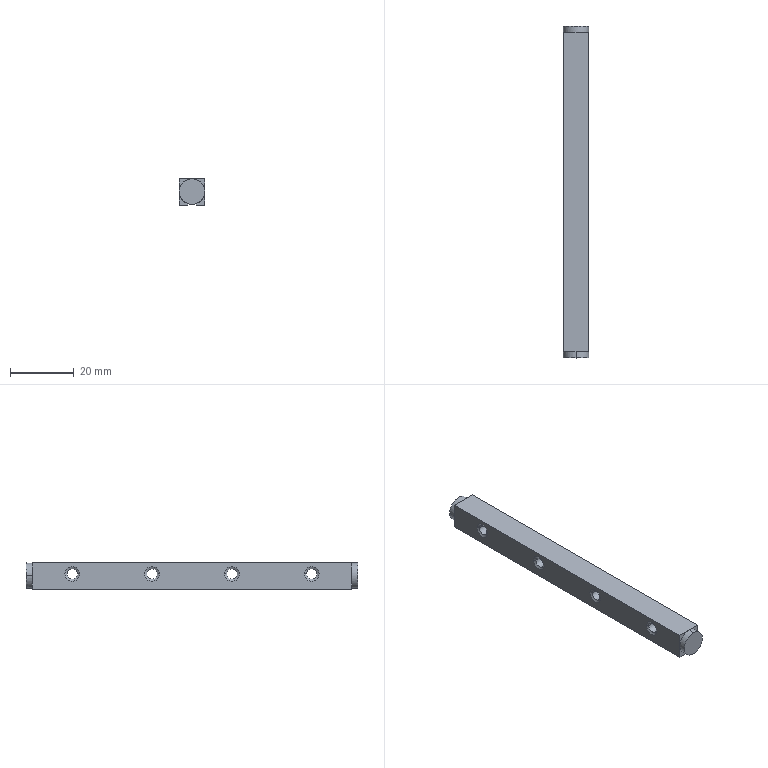Part | NX | 1 solid | 51 faces | box 8 x 104 x 8.3 mm | volume 6115 mm3 | plane 23 | cylinder 20 | cone 8 | commonest cylinder face diameters 3.3 x8 6 x8 8 x4
STEP:
#1=CARTESIAN_POINT('',(4.995,0.,-7.874));
#2=VERTEX_POINT('',#1);
#3=CARTESIAN_POINT('',(8.,0.,-4.));
#4=VERTEX_POINT('',#3);
#5=CARTESIAN_POINT('',(4.,0.,-4.));
#6=DIRECTION('',(0.,-1.,0.));
#7=DIRECTION('',(0.2489,0.,-0.9685));
#8=AXIS2_PLACEMENT_3D('',#5,#6,#7);
#9=CIRCLE('',#8,4.);
#10=EDGE_CURVE('',#2,#4,#9,.T.);
#11=ORIENTED_EDGE('',*,*,#10,.F.);
#12=CARTESIAN_POINT('',(5.421,0.,-8.3));
#13=VERTEX_POINT('',#12);
#14=CARTESIAN_POINT('',(5.421,0.,-8.3));
#15=DIRECTION('',(-0.7071,0.,0.7071));
#16=VECTOR('',#15,1000.);
#17=LINE('',#14,#16);
#18=EDGE_CURVE('',#13,#2,#17,.T.);
#19=ORIENTED_EDGE('',*,*,#18,.F.);
#20=CARTESIAN_POINT('',(8.,0.,-8.3));
#21=VERTEX_POINT('',#20);
#22=CARTESIAN_POINT('',(5.421,0.,-8.3));
#23=DIRECTION('',(1.,0.,0.));
#24=VECTOR('',#23,1000.);
#25=LINE('',#22,#24);
#26=EDGE_CURVE('',#13,#21,#25,.T.);
#27=ORIENTED_EDGE('',*,*,#26,.T.);
#28=CARTESIAN_POINT('',(8.,0.,-8.3));
#29=DIRECTION('',(0.,0.,1.));
#30=VECTOR('',#29,1000.);
#31=LINE('',#28,#30);
#32=EDGE_CURVE('',#21,#4,#31,.T.);
#33=ORIENTED_EDGE('',*,*,#32,.T.);
#34=EDGE_LOOP('',(#11,#19,#27,#33));
#35=FACE_BOUND('',#34,.T.);
#36=CARTESIAN_POINT('',(0.,0.,0.));
#37=DIRECTION('',(0.,1.,0.));
#38=DIRECTION('',(1.,0.,0.));
#39=AXIS2_PLACEMENT_3D('',#36,#37,#38);
#40=PLANE('',#39);
#41=ADVANCED_FACE('',(#35),#40,.F.);
#42=CARTESIAN_POINT('',(4.,-2.,0.));
#43=VERTEX_POINT('',#42);
#44=CARTESIAN_POINT('',(4.,-2.,-8.));
#45=VERTEX_POINT('',#44);
#46=CARTESIAN_POINT('',(4.,-2.,-4.));
#47=DIRECTION('',(0.,1.,0.));
#48=DIRECTION('',(0.,0.,1.));
#49=AXIS2_PLACEMENT_3D('',#46,#47,#48);
#50=CIRCLE('',#49,4.);
#51=EDGE_CURVE('',#43,#45,#50,.T.);
#52=ORIENTED_EDGE('',*,*,#51,.T.);
#53=CARTESIAN_POINT('',(4.,0.,-8.));
#54=VERTEX_POINT('',#53);
#55=CARTESIAN_POINT('',(4.,0.,-8.));
#56=DIRECTION('',(0.,-1.,0.));
#57=VECTOR('',#56,1000.);
#58=LINE('',#55,#57);
#59=EDGE_CURVE('',#45,#54,#58,.F.);
#60=ORIENTED_EDGE('',*,*,#59,.T.);
#61=CARTESIAN_POINT('',(4.,0.,-4.));
#62=DIRECTION('',(0.,-1.,0.));
#63=DIRECTION('',(-0.2489,0.,-0.9685));
#64=AXIS2_PLACEMENT_3D('',#61,#62,#63);
#65=CIRCLE('',#64,4.);
#66=EDGE_CURVE('',#54,#2,#65,.T.);
#67=ORIENTED_EDGE('',*,*,#66,.T.);
#68=ORIENTED_EDGE('',*,*,#10,.T.);
#69=CARTESIAN_POINT('',(4.,0.,0.));
#70=VERTEX_POINT('',#69);
#71=CARTESIAN_POINT('',(4.,0.,-4.));
#72=DIRECTION('',(0.,-1.,0.));
#73=DIRECTION('',(1.,0.,0.));
#74=AXIS2_PLACEMENT_3D('',#71,#72,#73);
#75=CIRCLE('',#74,4.);
#76=EDGE_CURVE('',#4,#70,#75,.T.);
#77=ORIENTED_EDGE('',*,*,#76,.T.);
#78=CARTESIAN_POINT('',(4.,0.,0.));
#79=DIRECTION('',(0.,-1.,0.));
#80=VECTOR('',#79,1000.);
#81=LINE('',#78,#80);
#82=EDGE_CURVE('',#43,#70,#81,.F.);
#83=ORIENTED_EDGE('',*,*,#82,.F.);
#84=EDGE_LOOP('',(#52,#60,#67,#68,#77,#83));
#85=FACE_BOUND('',#84,.T.);
#86=CARTESIAN_POINT('',(4.,0.,-4.));
#87=DIRECTION('',(0.,-1.,0.));
#88=DIRECTION('',(0.,0.,-1.));
#89=AXIS2_PLACEMENT_3D('',#86,#87,#88);
#90=CYLINDRICAL_SURFACE('',#89,4.);
#91=ADVANCED_FACE('',(#85),#90,.T.);
#92=CARTESIAN_POINT('',(4.,0.,-6.879));
#93=VERTEX_POINT('',#92);
#94=CARTESIAN_POINT('',(3.005,0.,-7.874));
#95=VERTEX_POINT('',#94);
#96=CARTESIAN_POINT('',(4.,0.,-6.879));
#97=DIRECTION('',(-0.7071,0.,-0.7071));
#98=VECTOR('',#97,1000.);
#99=LINE('',#96,#98);
#100=EDGE_CURVE('',#93,#95,#99,.T.);
#101=ORIENTED_EDGE('',*,*,#100,.F.);
#102=CARTESIAN_POINT('',(4.995,0.,-7.874));
#103=DIRECTION('',(-0.7071,0.,0.7071));
#104=VECTOR('',#103,1000.);
#105=LINE('',#102,#104);
#106=EDGE_CURVE('',#2,#93,#105,.T.);
#107=ORIENTED_EDGE('',*,*,#106,.F.);
#108=ORIENTED_EDGE('',*,*,#66,.F.);
#109=CARTESIAN_POINT('',(4.,0.,-4.));
#110=DIRECTION('',(0.,-1.,0.));
#111=DIRECTION('',(-0.2489,0.,-0.9685));
#112=AXIS2_PLACEMENT_3D('',#109,#110,#111);
#113=CIRCLE('',#112,4.);
#114=EDGE_CURVE('',#95,#54,#113,.T.);
#115=ORIENTED_EDGE('',*,*,#114,.F.);
#116=EDGE_LOOP('',(#101,#107,#108,#115));
#117=FACE_BOUND('',#116,.T.);
#118=CARTESIAN_POINT('',(0.,0.,0.));
#119=DIRECTION('',(0.,-1.,0.));
#120=DIRECTION('',(0.,0.,-1.));
#121=AXIS2_PLACEMENT_3D('',#118,#119,#120);
#122=PLANE('',#121);
#123=ADVANCED_FACE('',(#117),#122,.F.);
#124=ORIENTED_EDGE('',*,*,#100,.T.);
#125=CARTESIAN_POINT('',(2.579,0.,-8.3));
#126=VERTEX_POINT('',#125);
#127=CARTESIAN_POINT('',(3.005,0.,-7.874));
#128=DIRECTION('',(-0.7071,0.,-0.7071));
#129=VECTOR('',#128,1000.);
#130=LINE('',#127,#129);
#131=EDGE_CURVE('',#95,#126,#130,.T.);
#132=ORIENTED_EDGE('',*,*,#131,.T.);
#133=CARTESIAN_POINT('',(2.579,100.,-8.3));
#134=VERTEX_POINT('',#133);
#135=CARTESIAN_POINT('',(2.579,100.,-8.3));
#136=DIRECTION('',(0.,-1.,0.));
#137=VECTOR('',#136,1000.);
#138=LINE('',#135,#137);
#139=EDGE_CURVE('',#134,#126,#138,.T.);
#140=ORIENTED_EDGE('',*,*,#139,.F.);
#141=CARTESIAN_POINT('',(3.005,100.,-7.874));
#142=VERTEX_POINT('',#141);
#143=CARTESIAN_POINT('',(2.579,100.,-8.3));
#144=DIRECTION('',(0.7071,0.,0.7071));
#145=VECTOR('',#144,1000.);
#146=LINE('',#143,#145);
#147=EDGE_CURVE('',#134,#142,#146,.T.);
#148=ORIENTED_EDGE('',*,*,#147,.T.);
#149=CARTESIAN_POINT('',(4.,100.,-6.879));
#150=VERTEX_POINT('',#149);
#151=CARTESIAN_POINT('',(3.005,100.,-7.874));
#152=DIRECTION('',(0.7071,0.,0.7071));
#153=VECTOR('',#152,1000.);
#154=LINE('',#151,#153);
#155=EDGE_CURVE('',#142,#150,#154,.T.);
#156=ORIENTED_EDGE('',*,*,#155,.T.);
#157=CARTESIAN_POINT('',(4.,0.,-6.879));
#158=DIRECTION('',(0.,1.,0.));
#159=VECTOR('',#158,1000.);
#160=LINE('',#157,#159);
#161=EDGE_CURVE('',#93,#150,#160,.T.);
#162=ORIENTED_EDGE('',*,*,#161,.F.);
#163=EDGE_LOOP('',(#124,#132,#140,#148,#156,#162));
#164=FACE_BOUND('',#163,.T.);
#165=CARTESIAN_POINT('',(1.879,100.,-9.));
#166=DIRECTION('',(-0.7071,0.,0.7071));
#167=DIRECTION('',(0.,1.,0.));
#168=AXIS2_PLACEMENT_3D('',#165,#166,#167);
#169=PLANE('',#168);
#170=ADVANCED_FACE('',(#164),#169,.F.);
#171=ORIENTED_EDGE('',*,*,#106,.T.);
#172=ORIENTED_EDGE('',*,*,#161,.T.);
#173=CARTESIAN_POINT('',(4.995,100.,-7.874));
#174=VERTEX_POINT('',#173);
#175=CARTESIAN_POINT('',(4.,100.,-6.879));
#176=DIRECTION('',(0.7071,0.,-0.7071));
#177=VECTOR('',#176,1000.);
#178=LINE('',#175,#177);
#179=EDGE_CURVE('',#150,#174,#178,.T.);
#180=ORIENTED_EDGE('',*,*,#179,.T.);
#181=CARTESIAN_POINT('',(5.421,100.,-8.3));
#182=VERTEX_POINT('',#181);
#183=CARTESIAN_POINT('',(4.995,100.,-7.874));
#184=DIRECTION('',(0.7071,0.,-0.7071));
#185=VECTOR('',#184,1000.);
#186=LINE('',#183,#185);
#187=EDGE_CURVE('',#174,#182,#186,.T.);
#188=ORIENTED_EDGE('',*,*,#187,.T.);
#189=CARTESIAN_POINT('',(5.421,100.,-8.3));
#190=DIRECTION('',(0.,-1.,0.));
#191=VECTOR('',#190,1000.);
#192=LINE('',#189,#191);
#193=EDGE_CURVE('',#182,#13,#192,.T.);
#194=ORIENTED_EDGE('',*,*,#193,.T.);
#195=ORIENTED_EDGE('',*,*,#18,.T.);
#196=EDGE_LOOP('',(#171,#172,#180,#188,#194,#195));
#197=FACE_BOUND('',#196,.T.);
#198=CARTESIAN_POINT('',(4.,100.,-6.879));
#199=DIRECTION('',(0.7071,0.,0.7071));
#200=DIRECTION('',(0.,-1.,0.));
#201=AXIS2_PLACEMENT_3D('',#198,#199,#200);
#202=PLANE('',#201);
#203=ADVANCED_FACE('',(#197),#202,.F.);
#204=ORIENTED_EDGE('',*,*,#193,.F.);
#205=CARTESIAN_POINT('',(8.,100.,-8.3));
#206=VERTEX_POINT('',#205);
#207=CARTESIAN_POINT('',(5.421,100.,-8.3));
#208=DIRECTION('',(1.,0.,0.));
#209=VECTOR('',#208,1000.);
#210=LINE('',#207,#209);
#211=EDGE_CURVE('',#182,#206,#210,.T.);
#212=ORIENTED_EDGE('',*,*,#211,.T.);
#213=CARTESIAN_POINT('',(8.,100.,-8.3));
#214=DIRECTION('',(0.,-1.,0.));
#215=VECTOR('',#214,1000.);
#216=LINE('',#213,#215);
#217=EDGE_CURVE('',#206,#21,#216,.T.);
#218=ORIENTED_EDGE('',*,*,#217,.T.);
#219=ORIENTED_EDGE('',*,*,#26,.F.);
#220=EDGE_LOOP('',(#204,#212,#218,#219));
#221=FACE_BOUND('',#220,.T.);
#222=CARTESIAN_POINT('',(8.,0.,-8.3));
#223=DIRECTION('',(0.,0.,-1.));
#224=DIRECTION('',(0.,-1.,0.));
#225=AXIS2_PLACEMENT_3D('',#222,#223,#224);
#226=PLANE('',#225);
#227=ADVANCED_FACE('',(#221),#226,.T.);
#228=CARTESIAN_POINT('',(8.,0.,0.));
#229=VERTEX_POINT('',#228);
#230=CARTESIAN_POINT('',(8.,0.,-4.));
#231=DIRECTION('',(0.,0.,1.));
#232=VECTOR('',#231,1000.);
#233=LINE('',#230,#232);
#234=EDGE_CURVE('',#4,#229,#233,.T.);
#235=ORIENTED_EDGE('',*,*,#234,.F.);
#236=ORIENTED_EDGE('',*,*,#32,.F.);
#237=ORIENTED_EDGE('',*,*,#217,.F.);
#238=CARTESIAN_POINT('',(8.,100.,-4.));
#239=VERTEX_POINT('',#238);
#240=CARTESIAN_POINT('',(8.,100.,-8.3));
#241=DIRECTION('',(0.,0.,1.));
#242=VECTOR('',#241,1000.);
#243=LINE('',#240,#242);
#244=EDGE_CURVE('',#206,#239,#243,.T.);
#245=ORIENTED_EDGE('',*,*,#244,.T.);
#246=CARTESIAN_POINT('',(8.,100.,0.));
#247=VERTEX_POINT('',#246);
#248=CARTESIAN_POINT('',(8.,100.,-4.));
#249=DIRECTION('',(0.,0.,1.));
#250=VECTOR('',#249,1000.);
#251=LINE('',#248,#250);
#252=EDGE_CURVE('',#239,#247,#251,.T.);
#253=ORIENTED_EDGE('',*,*,#252,.T.);
#254=CARTESIAN_POINT('',(8.,100.,0.));
#255=DIRECTION('',(0.,-1.,0.));
#256=VECTOR('',#255,1000.);
#257=LINE('',#254,#256);
#258=EDGE_CURVE('',#247,#229,#257,.T.);
#259=ORIENTED_EDGE('',*,*,#258,.T.);
#260=EDGE_LOOP('',(#235,#236,#237,#245,#253,#259));
#261=FACE_BOUND('',#260,.T.);
#262=CARTESIAN_POINT('',(8.,84.5,-3.5));
#263=VERTEX_POINT('',#262);
#264=CARTESIAN_POINT('',(8.,90.5,-3.5));
#265=VERTEX_POINT('',#264);
#266=CARTESIAN_POINT('',(8.,87.5,-3.5));
#267=DIRECTION('',(1.,0.,0.));
#268=DIRECTION('',(0.,1.,0.));
#269=AXIS2_PLACEMENT_3D('',#266,#267,#268);
#270=CIRCLE('',#269,3.);
#271=EDGE_CURVE('',#263,#265,#270,.T.);
#272=ORIENTED_EDGE('',*,*,#271,.F.);
#273=CARTESIAN_POINT('',(8.,87.5,-3.5));
#274=DIRECTION('',(1.,0.,0.));
#275=DIRECTION('',(0.,1.,0.));
#276=AXIS2_PLACEMENT_3D('',#273,#274,#275);
#277=CIRCLE('',#276,3.);
#278=EDGE_CURVE('',#265,#263,#277,.T.);
#279=ORIENTED_EDGE('',*,*,#278,.F.);
#280=EDGE_LOOP('',(#272,#279));
#281=FACE_BOUND('',#280,.T.);
#282=CARTESIAN_POINT('',(8.,59.5,-3.5));
#283=VERTEX_POINT('',#282);
#284=CARTESIAN_POINT('',(8.,65.5,-3.5));
#285=VERTEX_POINT('',#284);
#286=CARTESIAN_POINT('',(8.,62.5,-3.5));
#287=DIRECTION('',(1.,0.,0.));
#288=DIRECTION('',(0.,1.,0.));
#289=AXIS2_PLACEMENT_3D('',#286,#287,#288);
#290=CIRCLE('',#289,3.);
#291=EDGE_CURVE('',#283,#285,#290,.T.);
#292=ORIENTED_EDGE('',*,*,#291,.F.);
#293=CARTESIAN_POINT('',(8.,62.5,-3.5));
#294=DIRECTION('',(1.,0.,0.));
#295=DIRECTION('',(0.,1.,0.));
#296=AXIS2_PLACEMENT_3D('',#293,#294,#295);
#297=CIRCLE('',#296,3.);
#298=EDGE_CURVE('',#285,#283,#297,.T.);
#299=ORIENTED_EDGE('',*,*,#298,.F.);
#300=EDGE_LOOP('',(#292,#299));
#301=FACE_BOUND('',#300,.T.);
#302=CARTESIAN_POINT('',(8.,40.5,-3.5));
#303=VERTEX_POINT('',#302);
#304=CARTESIAN_POINT('',(8.,34.5,-3.5));
#305=VERTEX_POINT('',#304);
#306=CARTESIAN_POINT('',(8.,37.5,-3.5));
#307=DIRECTION('',(1.,0.,0.));
#308=DIRECTION('',(0.,1.,0.));
#309=AXIS2_PLACEMENT_3D('',#306,#307,#308);
#310=CIRCLE('',#309,3.);
#311=EDGE_CURVE('',#303,#305,#310,.T.);
#312=ORIENTED_EDGE('',*,*,#311,.F.);
#313=CARTESIAN_POINT('',(8.,37.5,-3.5));
#314=DIRECTION('',(1.,0.,0.));
#315=DIRECTION('',(0.,1.,0.));
#316=AXIS2_PLACEMENT_3D('',#313,#314,#315);
#317=CIRCLE('',#316,3.);
#318=EDGE_CURVE('',#305,#303,#317,.T.);
#319=ORIENTED_EDGE('',*,*,#318,.F.);
#320=EDGE_LOOP('',(#312,#319));
#321=FACE_BOUND('',#320,.T.);
#322=CARTESIAN_POINT('',(8.,15.5,-3.5));
#323=VERTEX_POINT('',#322);
#324=CARTESIAN_POINT('',(8.,9.5,-3.5));
#325=VERTEX_POINT('',#324);
#326=CARTESIAN_POINT('',(8.,12.5,-3.5));
#327=DIRECTION('',(1.,0.,0.));
#328=DIRECTION('',(0.,1.,0.));
#329=AXIS2_PLACEMENT_3D('',#326,#327,#328);
#330=CIRCLE('',#329,3.);
#331=EDGE_CURVE('',#323,#325,#330,.T.);
#332=ORIENTED_EDGE('',*,*,#331,.F.);
#333=CARTESIAN_POINT('',(8.,12.5,-3.5));
#334=DIRECTION('',(1.,0.,0.));
#335=DIRECTION('',(0.,1.,0.));
#336=AXIS2_PLACEMENT_3D('',#333,#334,#335);
#337=CIRCLE('',#336,3.);
#338=EDGE_CURVE('',#325,#323,#337,.T.);
#339=ORIENTED_EDGE('',*,*,#338,.F.);
#340=EDGE_LOOP('',(#332,#339));
#341=FACE_BOUND('',#340,.T.);
#342=CARTESIAN_POINT('',(8.,0.,0.));
#343=DIRECTION('',(1.,0.,0.));
#344=DIRECTION('',(0.,1.,0.));
#345=AXIS2_PLACEMENT_3D('',#342,#343,#344);
#346=PLANE('',#345);
#347=ADVANCED_FACE('',(#261,#281,#301,#321,#341),#346,.T.);
#348=ORIENTED_EDGE('',*,*,#76,.F.);
#349=ORIENTED_EDGE('',*,*,#234,.T.);
#350=CARTESIAN_POINT('',(8.,0.,0.));
#351=DIRECTION('',(-1.,0.,0.));
#352=VECTOR('',#351,1000.);
#353=LINE('',#350,#352);
#354=EDGE_CURVE('',#229,#70,#353,.T.);
#355=ORIENTED_EDGE('',*,*,#354,.T.);
#356=EDGE_LOOP('',(#348,#349,#355));
#357=FACE_BOUND('',#356,.T.);
#358=CARTESIAN_POINT('',(0.,0.,0.));
#359=DIRECTION('',(0.,1.,0.));
#360=DIRECTION('',(1.,0.,0.));
#361=AXIS2_PLACEMENT_3D('',#358,#359,#360);
#362=PLANE('',#361);
#363=ADVANCED_FACE('',(#357),#362,.F.);
#364=CARTESIAN_POINT('',(0.,0.,0.));
#365=VERTEX_POINT('',#364);
#366=CARTESIAN_POINT('',(4.,0.,0.));
#367=DIRECTION('',(-1.,0.,0.));
#368=VECTOR('',#367,1000.);
#369=LINE('',#366,#368);
#370=EDGE_CURVE('',#70,#365,#369,.T.);
#371=ORIENTED_EDGE('',*,*,#370,.F.);
#372=ORIENTED_EDGE('',*,*,#354,.F.);
#373=ORIENTED_EDGE('',*,*,#258,.F.);
#374=CARTESIAN_POINT('',(4.,100.,0.));
#375=VERTEX_POINT('',#374);
#376=CARTESIAN_POINT('',(8.,100.,0.));
#377=DIRECTION('',(-1.,0.,0.));
#378=VECTOR('',#377,1000.);
#379=LINE('',#376,#378);
#380=EDGE_CURVE('',#247,#375,#379,.T.);
#381=ORIENTED_EDGE('',*,*,#380,.T.);
#382=CARTESIAN_POINT('',(0.,100.,0.));
#383=VERTEX_POINT('',#382);
#384=CARTESIAN_POINT('',(4.,100.,0.));
#385=DIRECTION('',(-1.,0.,0.));
#386=VECTOR('',#385,1000.);
#387=LINE('',#384,#386);
#388=EDGE_CURVE('',#375,#383,#387,.T.);
#389=ORIENTED_EDGE('',*,*,#388,.T.);
#390=CARTESIAN_POINT('',(0.,0.,0.));
#391=DIRECTION('',(0.,-1.,0.));
#392=VECTOR('',#391,1000.);
#393=LINE('',#390,#392);
#394=EDGE_CURVE('',#383,#365,#393,.T.);
#395=ORIENTED_EDGE('',*,*,#394,.T.);
#396=EDGE_LOOP('',(#371,#372,#373,#381,#389,#395));
#397=FACE_BOUND('',#396,.T.);
#398=CARTESIAN_POINT('',(0.,0.,0.));
#399=DIRECTION('',(0.,0.,1.));
#400=DIRECTION('',(1.,0.,0.));
#401=AXIS2_PLACEMENT_3D('',#398,#399,#400);
#402=PLANE('',#401);
#403=ADVANCED_FACE('',(#397),#402,.T.);
#404=CARTESIAN_POINT('',(0.,0.,-4.));
#405=VERTEX_POINT('',#404);
#406=CARTESIAN_POINT('',(4.,0.,-4.));
#407=DIRECTION('',(0.,-1.,0.));
#408=DIRECTION('',(0.,0.,1.));
#409=AXIS2_PLACEMENT_3D('',#406,#407,#408);
#410=CIRCLE('',#409,4.);
#411=EDGE_CURVE('',#70,#405,#410,.T.);
#412=ORIENTED_EDGE('',*,*,#411,.F.);
#413=ORIENTED_EDGE('',*,*,#370,.T.);
#414=CARTESIAN_POINT('',(0.,0.,0.));
#415=DIRECTION('',(0.,0.,1.));
#416=VECTOR('',#415,1000.);
#417=LINE('',#414,#416);
#418=EDGE_CURVE('',#405,#365,#417,.T.);
#419=ORIENTED_EDGE('',*,*,#418,.F.);
#420=EDGE_LOOP('',(#412,#413,#419));
#421=FACE_BOUND('',#420,.T.);
#422=CARTESIAN_POINT('',(0.,0.,0.));
#423=DIRECTION('',(0.,1.,0.));
#424=DIRECTION('',(1.,0.,0.));
#425=AXIS2_PLACEMENT_3D('',#422,#423,#424);
#426=PLANE('',#425);
#427=ADVANCED_FACE('',(#421),#426,.F.);
#428=CARTESIAN_POINT('',(4.9,15.5,-3.5));
#429=VERTEX_POINT('',#428);
#430=CARTESIAN_POINT('',(4.9,9.5,-3.5));
#431=VERTEX_POINT('',#430);
#432=CARTESIAN_POINT('',(4.9,12.5,-3.5));
#433=DIRECTION('',(1.,0.,0.));
#434=DIRECTION('',(0.,-1.,0.));
#435=AXIS2_PLACEMENT_3D('',#432,#433,#434);
#436=CIRCLE('',#435,3.);
#437=EDGE_CURVE('',#429,#431,#436,.T.);
#438=ORIENTED_EDGE('',*,*,#437,.T.);
#439=CARTESIAN_POINT('',(4.9,12.5,-3.5));
#440=DIRECTION('',(1.,0.,0.));
#441=DIRECTION('',(0.,-1.,0.));
#442=AXIS2_PLACEMENT_3D('',#439,#440,#441);
#443=CIRCLE('',#442,3.);
#444=EDGE_CURVE('',#431,#429,#443,.T.);
#445=ORIENTED_EDGE('',*,*,#444,.T.);
#446=EDGE_LOOP('',(#438,#445));
#447=FACE_BOUND('',#446,.T.);
#448=CARTESIAN_POINT('',(4.9,14.15,-3.5));
#449=VERTEX_POINT('',#448);
#450=CARTESIAN_POINT('',(4.9,10.85,-3.5));
#451=VERTEX_POINT('',#450);
#452=CARTESIAN_POINT('',(4.9,12.5,-3.5));
#453=DIRECTION('',(-1.,0.,0.));
#454=DIRECTION('',(0.,1.,0.));
#455=AXIS2_PLACEMENT_3D('',#452,#453,#454);
#456=CIRCLE('',#455,1.65);
#457=EDGE_CURVE('',#449,#451,#456,.T.);
#458=ORIENTED_EDGE('',*,*,#457,.T.);
#459=CARTESIAN_POINT('',(4.9,12.5,-3.5));
#460=DIRECTION('',(-1.,0.,0.));
#461=DIRECTION('',(0.,1.,0.));
#462=AXIS2_PLACEMENT_3D('',#459,#460,#461);
#463=CIRCLE('',#462,1.65);
#464=EDGE_CURVE('',#451,#449,#463,.T.);
#465=ORIENTED_EDGE('',*,*,#464,.T.);
#466=EDGE_LOOP('',(#458,#465));
#467=FACE_BOUND('',#466,.T.);
#468=CARTESIAN_POINT('',(4.9,12.5,-3.5));
#469=DIRECTION('',(1.,0.,0.));
#470=DIRECTION('',(0.,1.,0.));
#471=AXIS2_PLACEMENT_3D('',#468,#469,#470);
#472=PLANE('',#471);
#473=ADVANCED_FACE('',(#447,#467),#472,.T.);
#474=ORIENTED_EDGE('',*,*,#51,.F.);
#475=CARTESIAN_POINT('',(4.,-2.,-4.));
#476=DIRECTION('',(0.,1.,0.));
#477=DIRECTION('',(0.,0.,1.));
#478=AXIS2_PLACEMENT_3D('',#475,#476,#477);
#479=CIRCLE('',#478,4.);
#480=EDGE_CURVE('',#45,#43,#479,.T.);
#481=ORIENTED_EDGE('',*,*,#480,.F.);
#482=EDGE_LOOP('',(#474,#481));
#483=FACE_BOUND('',#482,.T.);
#484=CARTESIAN_POINT('',(0.,-2.,0.));
#485=DIRECTION('',(0.,-1.,0.));
#486=DIRECTION('',(0.,0.,-1.));
#487=AXIS2_PLACEMENT_3D('',#484,#485,#486);
#488=PLANE('',#487);
#489=ADVANCED_FACE('',(#483),#488,.T.);
#490=CARTESIAN_POINT('',(4.,0.,-4.));
#491=DIRECTION('',(0.,-1.,0.));
#492=DIRECTION('',(-1.,0.,0.));
#493=AXIS2_PLACEMENT_3D('',#490,#491,#492);
#494=CIRCLE('',#493,4.);
#495=EDGE_CURVE('',#405,#95,#494,.T.);
#496=ORIENTED_EDGE('',*,*,#495,.F.);
#497=CARTESIAN_POINT('',(0.,0.,-8.3));
#498=VERTEX_POINT('',#497);
#499=CARTESIAN_POINT('',(0.,0.,0.));
#500=DIRECTION('',(0.,0.,1.));
#501=VECTOR('',#500,1000.);
#502=LINE('',#499,#501);
#503=EDGE_CURVE('',#498,#405,#502,.T.);
#504=ORIENTED_EDGE('',*,*,#503,.F.);
#505=CARTESIAN_POINT('',(0.,0.,-8.3));
#506=DIRECTION('',(1.,0.,0.));
#507=VECTOR('',#506,1000.);
#508=LINE('',#505,#507);
#509=EDGE_CURVE('',#498,#126,#508,.T.);
#510=ORIENTED_EDGE('',*,*,#509,.T.);
#511=ORIENTED_EDGE('',*,*,#131,.F.);
#512=EDGE_LOOP('',(#496,#504,#510,#511));
#513=FACE_BOUND('',#512,.T.);
#514=CARTESIAN_POINT('',(0.,0.,0.));
#515=DIRECTION('',(0.,1.,0.));
#516=DIRECTION('',(1.,0.,0.));
#517=AXIS2_PLACEMENT_3D('',#514,#515,#516);
#518=PLANE('',#517);
#519=ADVANCED_FACE('',(#513),#518,.F.);
#520=ORIENTED_EDGE('',*,*,#139,.T.);
#521=ORIENTED_EDGE('',*,*,#509,.F.);
#522=CARTESIAN_POINT('',(0.,100.,-8.3));
#523=VERTEX_POINT('',#522);
#524=CARTESIAN_POINT('',(0.,0.,-8.3));
#525=DIRECTION('',(0.,1.,0.));
#526=VECTOR('',#525,1000.);
#527=LINE('',#524,#526);
#528=EDGE_CURVE('',#498,#523,#527,.T.);
#529=ORIENTED_EDGE('',*,*,#528,.T.);
#530=CARTESIAN_POINT('',(0.,100.,-8.3));
#531=DIRECTION('',(1.,0.,0.));
#532=VECTOR('',#531,1000.);
#533=LINE('',#530,#532);
#534=EDGE_CURVE('',#523,#134,#533,.T.);
#535=ORIENTED_EDGE('',*,*,#534,.T.);
#536=EDGE_LOOP('',(#520,#521,#529,#535));
#537=FACE_BOUND('',#536,.T.);
#538=CARTESIAN_POINT('',(8.,0.,-8.3));
#539=DIRECTION('',(0.,0.,-1.));
#540=DIRECTION('',(0.,-1.,0.));
#541=AXIS2_PLACEMENT_3D('',#538,#539,#540);
#542=PLANE('',#541);
#543=ADVANCED_FACE('',(#537),#542,.T.);
#544=CARTESIAN_POINT('',(0.,100.,-4.));
#545=VERTEX_POINT('',#544);
#546=CARTESIAN_POINT('',(4.,100.,-4.));
#547=DIRECTION('',(0.,1.,0.));
#548=DIRECTION('',(-0.2489,0.,-0.9685));
#549=AXIS2_PLACEMENT_3D('',#546,#547,#548);
#550=CIRCLE('',#549,4.);
#551=EDGE_CURVE('',#142,#545,#550,.T.);
#552=ORIENTED_EDGE('',*,*,#551,.F.);
#553=ORIENTED_EDGE('',*,*,#147,.F.);
#554=ORIENTED_EDGE('',*,*,#534,.F.);
#555=CARTESIAN_POINT('',(0.,100.,0.));
#556=DIRECTION('',(0.,0.,1.));
#557=VECTOR('',#556,1000.);
#558=LINE('',#555,#557);
#559=EDGE_CURVE('',#523,#545,#558,.T.);
#560=ORIENTED_EDGE('',*,*,#559,.T.);
#561=EDGE_LOOP('',(#552,#553,#554,#560));
#562=FACE_BOUND('',#561,.T.);
#563=CARTESIAN_POINT('',(0.,100.,0.));
#564=DIRECTION('',(0.,1.,0.));
#565=DIRECTION('',(1.,0.,0.));
#566=AXIS2_PLACEMENT_3D('',#563,#564,#565);
#567=PLANE('',#566);
#568=ADVANCED_FACE('',(#562),#567,.T.);
#569=CARTESIAN_POINT('',(8.,102.,-4.));
#570=VERTEX_POINT('',#569);
#571=CARTESIAN_POINT('',(0.,102.,-4.));
#572=VERTEX_POINT('',#571);
#573=CARTESIAN_POINT('',(4.,102.,-4.));
#574=DIRECTION('',(0.,-1.,0.));
#575=DIRECTION('',(1.,0.,0.));
#576=AXIS2_PLACEMENT_3D('',#573,#574,#575);
#577=CIRCLE('',#576,4.);
#578=EDGE_CURVE('',#570,#572,#577,.T.);
#579=ORIENTED_EDGE('',*,*,#578,.T.);
#580=CARTESIAN_POINT('',(0.,100.,-4.));
#581=DIRECTION('',(0.,1.,0.));
#582=VECTOR('',#581,1000.);
#583=LINE('',#580,#582);
#584=EDGE_CURVE('',#572,#545,#583,.F.);
#585=ORIENTED_EDGE('',*,*,#584,.T.);
#586=CARTESIAN_POINT('',(4.,100.,-4.));
#587=DIRECTION('',(0.,1.,0.));
#588=DIRECTION('',(-1.,0.,0.));
#589=AXIS2_PLACEMENT_3D('',#586,#587,#588);
#590=CIRCLE('',#589,4.);
#591=EDGE_CURVE('',#545,#375,#590,.T.);
#592=ORIENTED_EDGE('',*,*,#591,.T.);
#593=CARTESIAN_POINT('',(4.,100.,-4.));
#594=DIRECTION('',(0.,1.,0.));
#595=DIRECTION('',(0.,0.,1.));
#596=AXIS2_PLACEMENT_3D('',#593,#594,#595);
#597=CIRCLE('',#596,4.);
#598=EDGE_CURVE('',#375,#239,#597,.T.);
#599=ORIENTED_EDGE('',*,*,#598,.T.);
#600=CARTESIAN_POINT('',(8.,100.,-4.));
#601=DIRECTION('',(0.,1.,0.));
#602=VECTOR('',#601,1000.);
#603=LINE('',#600,#602);
#604=EDGE_CURVE('',#570,#239,#603,.F.);
#605=ORIENTED_EDGE('',*,*,#604,.F.);
#606=EDGE_LOOP('',(#579,#585,#592,#599,#605));
#607=FACE_BOUND('',#606,.T.);
#608=CARTESIAN_POINT('',(4.,100.,-4.));
#609=DIRECTION('',(0.,1.,0.));
#610=DIRECTION('',(-1.,0.,0.));
#611=AXIS2_PLACEMENT_3D('',#608,#609,#610);
#612=CYLINDRICAL_SURFACE('',#611,4.);
#613=ADVANCED_FACE('',(#607),#612,.T.);
#614=CARTESIAN_POINT('',(4.,100.,-4.));
#615=DIRECTION('',(0.,1.,0.));
#616=DIRECTION('',(1.,0.,0.));
#617=AXIS2_PLACEMENT_3D('',#614,#615,#616);
#618=CIRCLE('',#617,4.);
#619=EDGE_CURVE('',#239,#174,#618,.T.);
#620=ORIENTED_EDGE('',*,*,#619,.F.);
#621=ORIENTED_EDGE('',*,*,#244,.F.);
#622=ORIENTED_EDGE('',*,*,#211,.F.);
#623=ORIENTED_EDGE('',*,*,#187,.F.);
#624=EDGE_LOOP('',(#620,#621,#622,#623));
#625=FACE_BOUND('',#624,.T.);
#626=CARTESIAN_POINT('',(0.,100.,0.));
#627=DIRECTION('',(0.,1.,0.));
#628=DIRECTION('',(1.,0.,0.));
#629=AXIS2_PLACEMENT_3D('',#626,#627,#628);
#630=PLANE('',#629);
#631=ADVANCED_FACE('',(#625),#630,.T.);
#632=CARTESIAN_POINT('',(4.9,40.5,-3.5));
#633=VERTEX_POINT('',#632);
#634=CARTESIAN_POINT('',(4.9,34.5,-3.5));
#635=VERTEX_POINT('',#634);
#636=CARTESIAN_POINT('',(4.9,37.5,-3.5));
#637=DIRECTION('',(1.,0.,0.));
#638=DIRECTION('',(0.,-1.,0.));
#639=AXIS2_PLACEMENT_3D('',#636,#637,#638);
#640=CIRCLE('',#639,3.);
#641=EDGE_CURVE('',#633,#635,#640,.T.);
#642=ORIENTED_EDGE('',*,*,#641,.F.);
#643=CARTESIAN_POINT('',(-1.24,40.5,-3.5));
#644=DIRECTION('',(1.,0.,0.));
#645=VECTOR('',#644,1000.);
#646=LINE('',#643,#645);
#647=EDGE_CURVE('',#303,#633,#646,.F.);
#648=ORIENTED_EDGE('',*,*,#647,.F.);
#649=ORIENTED_EDGE('',*,*,#311,.T.);
#650=CARTESIAN_POINT('',(-1.24,34.5,-3.5));
#651=DIRECTION('',(1.,0.,0.));
#652=VECTOR('',#651,1000.);
#653=LINE('',#650,#652);
#654=EDGE_CURVE('',#305,#635,#653,.F.);
#655=ORIENTED_EDGE('',*,*,#654,.T.);
#656=EDGE_LOOP('',(#642,#648,#649,#655));
#657=FACE_BOUND('',#656,.T.);
#658=CARTESIAN_POINT('',(-1.24,37.5,-3.5));
#659=DIRECTION('',(1.,0.,0.));
#660=DIRECTION('',(0.,-1.,0.));
#661=AXIS2_PLACEMENT_3D('',#658,#659,#660);
#662=CYLINDRICAL_SURFACE('',#661,3.);
#663=ADVANCED_FACE('',(#657),#662,.F.);
#664=ORIENTED_EDGE('',*,*,#591,.F.);
#665=CARTESIAN_POINT('',(0.,100.,0.));
#666=DIRECTION('',(0.,0.,1.));
#667=VECTOR('',#666,1000.);
#668=LINE('',#665,#667);
#669=EDGE_CURVE('',#545,#383,#668,.T.);
#670=ORIENTED_EDGE('',*,*,#669,.T.);
#671=ORIENTED_EDGE('',*,*,#388,.F.);
#672=EDGE_LOOP('',(#664,#670,#671));
#673=FACE_BOUND('',#672,.T.);
#674=CARTESIAN_POINT('',(0.,100.,0.));
#675=DIRECTION('',(0.,1.,0.));
#676=DIRECTION('',(1.,0.,0.));
#677=AXIS2_PLACEMENT_3D('',#674,#675,#676);
#678=PLANE('',#677);
#679=ADVANCED_FACE('',(#673),#678,.T.);
#680=ORIENTED_EDGE('',*,*,#503,.T.);
#681=ORIENTED_EDGE('',*,*,#418,.T.);
#682=ORIENTED_EDGE('',*,*,#394,.F.);
#683=ORIENTED_EDGE('',*,*,#669,.F.);
#684=ORIENTED_EDGE('',*,*,#559,.F.);
#685=ORIENTED_EDGE('',*,*,#528,.F.);
#686=EDGE_LOOP('',(#680,#681,#682,#683,#684,#685));
#687=FACE_BOUND('',#686,.T.);
#688=CARTESIAN_POINT('',(0.,10.185,-3.5));
#689=VERTEX_POINT('',#688);
#690=CARTESIAN_POINT('',(0.,14.815,-3.5));
#691=VERTEX_POINT('',#690);
#692=CARTESIAN_POINT('',(0.,12.5,-3.5));
#693=DIRECTION('',(-1.,0.,0.));
#694=DIRECTION('',(0.,1.,0.));
#695=AXIS2_PLACEMENT_3D('',#692,#693,#694);
#696=CIRCLE('',#695,2.315);
#697=EDGE_CURVE('',#689,#691,#696,.T.);
#698=ORIENTED_EDGE('',*,*,#697,.F.);
#699=CARTESIAN_POINT('',(0.,12.5,-3.5));
#700=DIRECTION('',(-1.,0.,0.));
#701=DIRECTION('',(0.,1.,0.));
#702=AXIS2_PLACEMENT_3D('',#699,#700,#701);
#703=CIRCLE('',#702,2.315);
#704=EDGE_CURVE('',#691,#689,#703,.T.);
#705=ORIENTED_EDGE('',*,*,#704,.F.);
#706=EDGE_LOOP('',(#698,#705));
#707=FACE_BOUND('',#706,.T.);
#708=CARTESIAN_POINT('',(0.,89.815,-3.5));
#709=VERTEX_POINT('',#708);
#710=CARTESIAN_POINT('',(0.,85.185,-3.5));
#711=VERTEX_POINT('',#710);
#712=CARTESIAN_POINT('',(0.,87.5,-3.5));
#713=DIRECTION('',(-1.,0.,0.));
#714=DIRECTION('',(0.,1.,0.));
#715=AXIS2_PLACEMENT_3D('',#712,#713,#714);
#716=CIRCLE('',#715,2.315);
#717=EDGE_CURVE('',#709,#711,#716,.T.);
#718=ORIENTED_EDGE('',*,*,#717,.F.);
#719=CARTESIAN_POINT('',(0.,87.5,-3.5));
#720=DIRECTION('',(-1.,0.,0.));
#721=DIRECTION('',(0.,1.,0.));
#722=AXIS2_PLACEMENT_3D('',#719,#720,#721);
#723=CIRCLE('',#722,2.315);
#724=EDGE_CURVE('',#711,#709,#723,.T.);
#725=ORIENTED_EDGE('',*,*,#724,.F.);
#726=EDGE_LOOP('',(#718,#725));
#727=FACE_BOUND('',#726,.T.);
#728=CARTESIAN_POINT('',(0.,35.185,-3.5));
#729=VERTEX_POINT('',#728);
#730=CARTESIAN_POINT('',(0.,39.815,-3.5));
#731=VERTEX_POINT('',#730);
#732=CARTESIAN_POINT('',(0.,37.5,-3.5));
#733=DIRECTION('',(-1.,0.,0.));
#734=DIRECTION('',(0.,1.,0.));
#735=AXIS2_PLACEMENT_3D('',#732,#733,#734);
#736=CIRCLE('',#735,2.315);
#737=EDGE_CURVE('',#729,#731,#736,.T.);
#738=ORIENTED_EDGE('',*,*,#737,.F.);
#739=CARTESIAN_POINT('',(0.,37.5,-3.5));
#740=DIRECTION('',(-1.,0.,0.));
#741=DIRECTION('',(0.,1.,0.));
#742=AXIS2_PLACEMENT_3D('',#739,#740,#741);
#743=CIRCLE('',#742,2.315);
#744=EDGE_CURVE('',#731,#729,#743,.T.);
#745=ORIENTED_EDGE('',*,*,#744,.F.);
#746=EDGE_LOOP('',(#738,#745));
#747=FACE_BOUND('',#746,.T.);
#748=CARTESIAN_POINT('',(0.,60.185,-3.5));
#749=VERTEX_POINT('',#748);
#750=CARTESIAN_POINT('',(0.,64.815,-3.5));
#751=VERTEX_POINT('',#750);
#752=CARTESIAN_POINT('',(0.,62.5,-3.5));
#753=DIRECTION('',(-1.,0.,0.));
#754=DIRECTION('',(0.,1.,0.));
#755=AXIS2_PLACEMENT_3D('',#752,#753,#754);
#756=CIRCLE('',#755,2.315);
#757=EDGE_CURVE('',#749,#751,#756,.T.);
#758=ORIENTED_EDGE('',*,*,#757,.F.);
#759=CARTESIAN_POINT('',(0.,62.5,-3.5));
#760=DIRECTION('',(-1.,0.,0.));
#761=DIRECTION('',(0.,1.,0.));
#762=AXIS2_PLACEMENT_3D('',#759,#760,#761);
#763=CIRCLE('',#762,2.315);
#764=EDGE_CURVE('',#751,#749,#763,.T.);
#765=ORIENTED_EDGE('',*,*,#764,.F.);
#766=EDGE_LOOP('',(#758,#765));
#767=FACE_BOUND('',#766,.T.);
#768=CARTESIAN_POINT('',(0.,0.,-8.3));
#769=DIRECTION('',(-1.,0.,0.));
#770=DIRECTION('',(0.,0.,1.));
#771=AXIS2_PLACEMENT_3D('',#768,#769,#770);
#772=PLANE('',#771);
#773=ADVANCED_FACE('',(#687,#707,#727,#747,#767),#772,.T.);
#774=ORIENTED_EDGE('',*,*,#578,.F.);
#775=CARTESIAN_POINT('',(4.,102.,-4.));
#776=DIRECTION('',(0.,-1.,0.));
#777=DIRECTION('',(1.,0.,0.));
#778=AXIS2_PLACEMENT_3D('',#775,#776,#777);
#779=CIRCLE('',#778,4.);
#780=EDGE_CURVE('',#572,#570,#779,.T.);
#781=ORIENTED_EDGE('',*,*,#780,.F.);
#782=EDGE_LOOP('',(#774,#781));
#783=FACE_BOUND('',#782,.T.);
#784=CARTESIAN_POINT('',(0.,102.,0.));
#785=DIRECTION('',(0.,1.,0.));
#786=DIRECTION('',(1.,0.,0.));
#787=AXIS2_PLACEMENT_3D('',#784,#785,#786);
#788=PLANE('',#787);
#789=ADVANCED_FACE('',(#783),#788,.T.);
#790=ORIENTED_EDGE('',*,*,#641,.T.);
#791=CARTESIAN_POINT('',(4.9,37.5,-3.5));
#792=DIRECTION('',(1.,0.,0.));
#793=DIRECTION('',(0.,-1.,0.));
#794=AXIS2_PLACEMENT_3D('',#791,#792,#793);
#795=CIRCLE('',#794,3.);
#796=EDGE_CURVE('',#635,#633,#795,.T.);
#797=ORIENTED_EDGE('',*,*,#796,.T.);
#798=EDGE_LOOP('',(#790,#797));
#799=FACE_BOUND('',#798,.T.);
#800=CARTESIAN_POINT('',(4.9,35.85,-3.5));
#801=VERTEX_POINT('',#800);
#802=CARTESIAN_POINT('',(4.9,39.15,-3.5));
#803=VERTEX_POINT('',#802);
#804=CARTESIAN_POINT('',(4.9,37.5,-3.5));
#805=DIRECTION('',(-1.,0.,0.));
#806=DIRECTION('',(0.,1.,0.));
#807=AXIS2_PLACEMENT_3D('',#804,#805,#806);
#808=CIRCLE('',#807,1.65);
#809=EDGE_CURVE('',#801,#803,#808,.T.);
#810=ORIENTED_EDGE('',*,*,#809,.T.);
#811=CARTESIAN_POINT('',(4.9,37.5,-3.5));
#812=DIRECTION('',(-1.,0.,0.));
#813=DIRECTION('',(0.,1.,0.));
#814=AXIS2_PLACEMENT_3D('',#811,#812,#813);
#815=CIRCLE('',#814,1.65);
#816=EDGE_CURVE('',#803,#801,#815,.T.);
#817=ORIENTED_EDGE('',*,*,#816,.T.);
#818=EDGE_LOOP('',(#810,#817));
#819=FACE_BOUND('',#818,.T.);
#820=CARTESIAN_POINT('',(4.9,37.5,-3.5));
#821=DIRECTION('',(1.,0.,0.));
#822=DIRECTION('',(0.,1.,0.));
#823=AXIS2_PLACEMENT_3D('',#820,#821,#822);
#824=PLANE('',#823);
#825=ADVANCED_FACE('',(#799,#819),#824,.T.);
#826=CARTESIAN_POINT('',(4.9,84.5,-3.5));
#827=VERTEX_POINT('',#826);
#828=CARTESIAN_POINT('',(4.9,90.5,-3.5));
#829=VERTEX_POINT('',#828);
#830=CARTESIAN_POINT('',(4.9,87.5,-3.5));
#831=DIRECTION('',(1.,0.,0.));
#832=DIRECTION('',(0.,-1.,0.));
#833=AXIS2_PLACEMENT_3D('',#830,#831,#832);
#834=CIRCLE('',#833,3.);
#835=EDGE_CURVE('',#827,#829,#834,.T.);
#836=ORIENTED_EDGE('',*,*,#835,.T.);
#837=CARTESIAN_POINT('',(4.9,87.5,-3.5));
#838=DIRECTION('',(1.,0.,0.));
#839=DIRECTION('',(0.,-1.,0.));
#840=AXIS2_PLACEMENT_3D('',#837,#838,#839);
#841=CIRCLE('',#840,3.);
#842=EDGE_CURVE('',#829,#827,#841,.T.);
#843=ORIENTED_EDGE('',*,*,#842,.T.);
#844=EDGE_LOOP('',(#836,#843));
#845=FACE_BOUND('',#844,.T.);
#846=CARTESIAN_POINT('',(4.9,89.15,-3.5));
#847=VERTEX_POINT('',#846);
#848=CARTESIAN_POINT('',(4.9,85.85,-3.5));
#849=VERTEX_POINT('',#848);
#850=CARTESIAN_POINT('',(4.9,87.5,-3.5));
#851=DIRECTION('',(-1.,0.,0.));
#852=DIRECTION('',(0.,1.,0.));
#853=AXIS2_PLACEMENT_3D('',#850,#851,#852);
#854=CIRCLE('',#853,1.65);
#855=EDGE_CURVE('',#847,#849,#854,.T.);
#856=ORIENTED_EDGE('',*,*,#855,.T.);
#857=CARTESIAN_POINT('',(4.9,87.5,-3.5));
#858=DIRECTION('',(-1.,0.,0.));
#859=DIRECTION('',(0.,1.,0.));
#860=AXIS2_PLACEMENT_3D('',#857,#858,#859);
#861=CIRCLE('',#860,1.65);
#862=EDGE_CURVE('',#849,#847,#861,.T.);
#863=ORIENTED_EDGE('',*,*,#862,.T.);
#864=EDGE_LOOP('',(#856,#863));
#865=FACE_BOUND('',#864,.T.);
#866=CARTESIAN_POINT('',(4.9,87.5,-3.5));
#867=DIRECTION('',(1.,0.,0.));
#868=DIRECTION('',(0.,1.,0.));
#869=AXIS2_PLACEMENT_3D('',#866,#867,#868);
#870=PLANE('',#869);
#871=ADVANCED_FACE('',(#845,#865),#870,.T.);
#872=ORIENTED_EDGE('',*,*,#271,.T.);
#873=CARTESIAN_POINT('',(-1.24,90.5,-3.5));
#874=DIRECTION('',(1.,0.,0.));
#875=VECTOR('',#874,1000.);
#876=LINE('',#873,#875);
#877=EDGE_CURVE('',#265,#829,#876,.F.);
#878=ORIENTED_EDGE('',*,*,#877,.T.);
#879=ORIENTED_EDGE('',*,*,#835,.F.);
#880=CARTESIAN_POINT('',(-1.24,84.5,-3.5));
#881=DIRECTION('',(1.,0.,0.));
#882=VECTOR('',#881,1000.);
#883=LINE('',#880,#882);
#884=EDGE_CURVE('',#263,#827,#883,.F.);
#885=ORIENTED_EDGE('',*,*,#884,.F.);
#886=EDGE_LOOP('',(#872,#878,#879,#885));
#887=FACE_BOUND('',#886,.T.);
#888=CARTESIAN_POINT('',(-1.24,87.5,-3.5));
#889=DIRECTION('',(1.,0.,0.));
#890=DIRECTION('',(0.,-1.,0.));
#891=AXIS2_PLACEMENT_3D('',#888,#889,#890);
#892=CYLINDRICAL_SURFACE('',#891,3.);
#893=ADVANCED_FACE('',(#887),#892,.F.);
#894=ORIENTED_EDGE('',*,*,#437,.F.);
#895=CARTESIAN_POINT('',(-1.24,15.5,-3.5));
#896=DIRECTION('',(1.,0.,0.));
#897=VECTOR('',#896,1000.);
#898=LINE('',#895,#897);
#899=EDGE_CURVE('',#323,#429,#898,.F.);
#900=ORIENTED_EDGE('',*,*,#899,.F.);
#901=ORIENTED_EDGE('',*,*,#331,.T.);
#902=CARTESIAN_POINT('',(-1.24,9.5,-3.5));
#903=DIRECTION('',(1.,0.,0.));
#904=VECTOR('',#903,1000.);
#905=LINE('',#902,#904);
#906=EDGE_CURVE('',#325,#431,#905,.F.);
#907=ORIENTED_EDGE('',*,*,#906,.T.);
#908=EDGE_LOOP('',(#894,#900,#901,#907));
#909=FACE_BOUND('',#908,.T.);
#910=CARTESIAN_POINT('',(-1.24,12.5,-3.5));
#911=DIRECTION('',(1.,0.,0.));
#912=DIRECTION('',(0.,-1.,0.));
#913=AXIS2_PLACEMENT_3D('',#910,#911,#912);
#914=CYLINDRICAL_SURFACE('',#913,3.);
#915=ADVANCED_FACE('',(#909),#914,.F.);
#916=ORIENTED_EDGE('',*,*,#155,.F.);
#917=CARTESIAN_POINT('',(4.,100.,-4.));
#918=DIRECTION('',(0.,1.,0.));
#919=DIRECTION('',(0.2489,0.,-0.9685));
#920=AXIS2_PLACEMENT_3D('',#917,#918,#919);
#921=CIRCLE('',#920,4.);
#922=EDGE_CURVE('',#174,#142,#921,.T.);
#923=ORIENTED_EDGE('',*,*,#922,.F.);
#924=ORIENTED_EDGE('',*,*,#179,.F.);
#925=EDGE_LOOP('',(#916,#923,#924));
#926=FACE_BOUND('',#925,.T.);
#927=CARTESIAN_POINT('',(0.,100.,0.));
#928=DIRECTION('',(0.,1.,0.));
#929=DIRECTION('',(1.,0.,0.));
#930=AXIS2_PLACEMENT_3D('',#927,#928,#929);
#931=PLANE('',#930);
#932=ADVANCED_FACE('',(#926),#931,.F.);
#933=ORIENTED_EDGE('',*,*,#598,.F.);
#934=ORIENTED_EDGE('',*,*,#380,.F.);
#935=ORIENTED_EDGE('',*,*,#252,.F.);
#936=EDGE_LOOP('',(#933,#934,#935));
#937=FACE_BOUND('',#936,.T.);
#938=CARTESIAN_POINT('',(0.,100.,0.));
#939=DIRECTION('',(0.,1.,0.));
#940=DIRECTION('',(1.,0.,0.));
#941=AXIS2_PLACEMENT_3D('',#938,#939,#940);
#942=PLANE('',#941);
#943=ADVANCED_FACE('',(#937),#942,.T.);
#944=CARTESIAN_POINT('',(4.9,59.5,-3.5));
#945=VERTEX_POINT('',#944);
#946=CARTESIAN_POINT('',(4.9,65.5,-3.5));
#947=VERTEX_POINT('',#946);
#948=CARTESIAN_POINT('',(4.9,62.5,-3.5));
#949=DIRECTION('',(1.,0.,0.));
#950=DIRECTION('',(0.,-1.,0.));
#951=AXIS2_PLACEMENT_3D('',#948,#949,#950);
#952=CIRCLE('',#951,3.);
#953=EDGE_CURVE('',#945,#947,#952,.T.);
#954=ORIENTED_EDGE('',*,*,#953,.T.);
#955=CARTESIAN_POINT('',(4.9,62.5,-3.5));
#956=DIRECTION('',(1.,0.,0.));
#957=DIRECTION('',(0.,-1.,0.));
#958=AXIS2_PLACEMENT_3D('',#955,#956,#957);
#959=CIRCLE('',#958,3.);
#960=EDGE_CURVE('',#947,#945,#959,.T.);
#961=ORIENTED_EDGE('',*,*,#960,.T.);
#962=EDGE_LOOP('',(#954,#961));
#963=FACE_BOUND('',#962,.T.);
#964=CARTESIAN_POINT('',(4.9,60.85,-3.5));
#965=VERTEX_POINT('',#964);
#966=CARTESIAN_POINT('',(4.9,64.15,-3.5));
#967=VERTEX_POINT('',#966);
#968=CARTESIAN_POINT('',(4.9,62.5,-3.5));
#969=DIRECTION('',(-1.,0.,0.));
#970=DIRECTION('',(0.,1.,0.));
#971=AXIS2_PLACEMENT_3D('',#968,#969,#970);
#972=CIRCLE('',#971,1.65);
#973=EDGE_CURVE('',#965,#967,#972,.T.);
#974=ORIENTED_EDGE('',*,*,#973,.T.);
#975=CARTESIAN_POINT('',(4.9,62.5,-3.5));
#976=DIRECTION('',(-1.,0.,0.));
#977=DIRECTION('',(0.,1.,0.));
#978=AXIS2_PLACEMENT_3D('',#975,#976,#977);
#979=CIRCLE('',#978,1.65);
#980=EDGE_CURVE('',#967,#965,#979,.T.);
#981=ORIENTED_EDGE('',*,*,#980,.T.);
#982=EDGE_LOOP('',(#974,#981));
#983=FACE_BOUND('',#982,.T.);
#984=CARTESIAN_POINT('',(4.9,62.5,-3.5));
#985=DIRECTION('',(1.,0.,0.));
#986=DIRECTION('',(0.,1.,0.));
#987=AXIS2_PLACEMENT_3D('',#984,#985,#986);
#988=PLANE('',#987);
#989=ADVANCED_FACE('',(#963,#983),#988,.T.);
#990=ORIENTED_EDGE('',*,*,#291,.T.);
#991=CARTESIAN_POINT('',(-1.24,65.5,-3.5));
#992=DIRECTION('',(1.,0.,0.));
#993=VECTOR('',#992,1000.);
#994=LINE('',#991,#993);
#995=EDGE_CURVE('',#285,#947,#994,.F.);
#996=ORIENTED_EDGE('',*,*,#995,.T.);
#997=ORIENTED_EDGE('',*,*,#953,.F.);
#998=CARTESIAN_POINT('',(-1.24,59.5,-3.5));
#999=DIRECTION('',(1.,0.,0.));
#1000=VECTOR('',#999,1000.);
#1001=LINE('',#998,#1000);
#1002=EDGE_CURVE('',#283,#945,#1001,.F.);
#1003=ORIENTED_EDGE('',*,*,#1002,.F.);
#1004=EDGE_LOOP('',(#990,#996,#997,#1003));
#1005=FACE_BOUND('',#1004,.T.);
#1006=CARTESIAN_POINT('',(-1.24,62.5,-3.5));
#1007=DIRECTION('',(1.,0.,0.));
#1008=DIRECTION('',(0.,-1.,0.));
#1009=AXIS2_PLACEMENT_3D('',#1006,#1007,#1008);
#1010=CYLINDRICAL_SURFACE('',#1009,3.);
#1011=ADVANCED_FACE('',(#1005),#1010,.F.);
#1012=ORIENTED_EDGE('',*,*,#457,.F.);
#1013=CARTESIAN_POINT('',(0.3839,14.15,-3.5));
#1014=VERTEX_POINT('',#1013);
#1015=CARTESIAN_POINT('',(0.,14.15,-3.5));
#1016=DIRECTION('',(-1.,0.,0.));
#1017=VECTOR('',#1016,1000.);
#1018=LINE('',#1015,#1017);
#1019=EDGE_CURVE('',#449,#1014,#1018,.T.);
#1020=ORIENTED_EDGE('',*,*,#1019,.T.);
#1021=CARTESIAN_POINT('',(0.3839,10.85,-3.5));
#1022=VERTEX_POINT('',#1021);
#1023=CARTESIAN_POINT('',(0.3839,12.5,-3.5));
#1024=DIRECTION('',(-1.,0.,0.));
#1025=DIRECTION('',(0.,1.,0.));
#1026=AXIS2_PLACEMENT_3D('',#1023,#1024,#1025);
#1027=CIRCLE('',#1026,1.65);
#1028=EDGE_CURVE('',#1014,#1022,#1027,.T.);
#1029=ORIENTED_EDGE('',*,*,#1028,.T.);
#1030=CARTESIAN_POINT('',(0.,10.85,-3.5));
#1031=DIRECTION('',(-1.,0.,0.));
#1032=VECTOR('',#1031,1000.);
#1033=LINE('',#1030,#1032);
#1034=EDGE_CURVE('',#451,#1022,#1033,.T.);
#1035=ORIENTED_EDGE('',*,*,#1034,.F.);
#1036=EDGE_LOOP('',(#1012,#1020,#1029,#1035));
#1037=FACE_BOUND('',#1036,.T.);
#1038=CARTESIAN_POINT('',(0.,12.5,-3.5));
#1039=DIRECTION('',(-1.,0.,0.));
#1040=DIRECTION('',(0.,1.,0.));
#1041=AXIS2_PLACEMENT_3D('',#1038,#1039,#1040);
#1042=CYLINDRICAL_SURFACE('',#1041,1.65);
#1043=ADVANCED_FACE('',(#1037),#1042,.F.);
#1044=ORIENTED_EDGE('',*,*,#697,.T.);
#1045=CARTESIAN_POINT('',(0.3839,14.15,-3.5));
#1046=DIRECTION('',(-0.5,0.866,0.));
#1047=VECTOR('',#1046,1000.);
#1048=LINE('',#1045,#1047);
#1049=EDGE_CURVE('',#1014,#691,#1048,.T.);
#1050=ORIENTED_EDGE('',*,*,#1049,.F.);
#1051=CARTESIAN_POINT('',(0.3839,12.5,-3.5));
#1052=DIRECTION('',(-1.,0.,0.));
#1053=DIRECTION('',(0.,1.,0.));
#1054=AXIS2_PLACEMENT_3D('',#1051,#1052,#1053);
#1055=CIRCLE('',#1054,1.65);
#1056=EDGE_CURVE('',#1022,#1014,#1055,.T.);
#1057=ORIENTED_EDGE('',*,*,#1056,.F.);
#1058=CARTESIAN_POINT('',(0.3839,10.85,-3.5));
#1059=DIRECTION('',(-0.5,-0.866,0.));
#1060=VECTOR('',#1059,1000.);
#1061=LINE('',#1058,#1060);
#1062=EDGE_CURVE('',#1022,#689,#1061,.T.);
#1063=ORIENTED_EDGE('',*,*,#1062,.T.);
#1064=EDGE_LOOP('',(#1044,#1050,#1057,#1063));
#1065=FACE_BOUND('',#1064,.T.);
#1066=CARTESIAN_POINT('',(0.3839,12.5,-3.5));
#1067=DIRECTION('',(-1.,0.,0.));
#1068=DIRECTION('',(0.,1.,0.));
#1069=AXIS2_PLACEMENT_3D('',#1066,#1067,#1068);
#1070=CONICAL_SURFACE('',#1069,1.65,1.047);
#1071=ADVANCED_FACE('',(#1065),#1070,.F.);
#1072=CARTESIAN_POINT('',(0.3839,39.15,-3.5));
#1073=VERTEX_POINT('',#1072);
#1074=CARTESIAN_POINT('',(0.3839,35.85,-3.5));
#1075=VERTEX_POINT('',#1074);
#1076=CARTESIAN_POINT('',(0.3839,37.5,-3.5));
#1077=DIRECTION('',(-1.,0.,0.));
#1078=DIRECTION('',(0.,1.,0.));
#1079=AXIS2_PLACEMENT_3D('',#1076,#1077,#1078);
#1080=CIRCLE('',#1079,1.65);
#1081=EDGE_CURVE('',#1073,#1075,#1080,.T.);
#1082=ORIENTED_EDGE('',*,*,#1081,.T.);
#1083=CARTESIAN_POINT('',(0.,35.85,-3.5));
#1084=DIRECTION('',(-1.,0.,0.));
#1085=VECTOR('',#1084,1000.);
#1086=LINE('',#1083,#1085);
#1087=EDGE_CURVE('',#1075,#801,#1086,.F.);
#1088=ORIENTED_EDGE('',*,*,#1087,.T.);
#1089=ORIENTED_EDGE('',*,*,#816,.F.);
#1090=CARTESIAN_POINT('',(0.,39.15,-3.5));
#1091=DIRECTION('',(-1.,0.,0.));
#1092=VECTOR('',#1091,1000.);
#1093=LINE('',#1090,#1092);
#1094=EDGE_CURVE('',#1073,#803,#1093,.F.);
#1095=ORIENTED_EDGE('',*,*,#1094,.F.);
#1096=EDGE_LOOP('',(#1082,#1088,#1089,#1095));
#1097=FACE_BOUND('',#1096,.T.);
#1098=CARTESIAN_POINT('',(0.,37.5,-3.5));
#1099=DIRECTION('',(-1.,0.,0.));
#1100=DIRECTION('',(0.,1.,0.));
#1101=AXIS2_PLACEMENT_3D('',#1098,#1099,#1100);
#1102=CYLINDRICAL_SURFACE('',#1101,1.65);
#1103=ADVANCED_FACE('',(#1097),#1102,.F.);
#1104=ORIENTED_EDGE('',*,*,#1081,.F.);
#1105=CARTESIAN_POINT('',(0.3839,39.15,-3.5));
#1106=DIRECTION('',(-0.5,0.866,0.));
#1107=VECTOR('',#1106,1000.);
#1108=LINE('',#1105,#1107);
#1109=EDGE_CURVE('',#1073,#731,#1108,.T.);
#1110=ORIENTED_EDGE('',*,*,#1109,.T.);
#1111=ORIENTED_EDGE('',*,*,#744,.T.);
#1112=CARTESIAN_POINT('',(0.3839,35.85,-3.5));
#1113=DIRECTION('',(-0.5,-0.866,0.));
#1114=VECTOR('',#1113,1000.);
#1115=LINE('',#1112,#1114);
#1116=EDGE_CURVE('',#1075,#729,#1115,.T.);
#1117=ORIENTED_EDGE('',*,*,#1116,.F.);
#1118=EDGE_LOOP('',(#1104,#1110,#1111,#1117));
#1119=FACE_BOUND('',#1118,.T.);
#1120=CARTESIAN_POINT('',(0.3839,37.5,-3.5));
#1121=DIRECTION('',(-1.,0.,0.));
#1122=DIRECTION('',(0.,1.,0.));
#1123=AXIS2_PLACEMENT_3D('',#1120,#1121,#1122);
#1124=CONICAL_SURFACE('',#1123,1.65,1.047);
#1125=ADVANCED_FACE('',(#1119),#1124,.F.);
#1126=ORIENTED_EDGE('',*,*,#973,.F.);
#1127=CARTESIAN_POINT('',(0.3839,60.85,-3.5));
#1128=VERTEX_POINT('',#1127);
#1129=CARTESIAN_POINT('',(0.,60.85,-3.5));
#1130=DIRECTION('',(-1.,0.,0.));
#1131=VECTOR('',#1130,1000.);
#1132=LINE('',#1129,#1131);
#1133=EDGE_CURVE('',#1128,#965,#1132,.F.);
#1134=ORIENTED_EDGE('',*,*,#1133,.F.);
#1135=CARTESIAN_POINT('',(0.3839,64.15,-3.5));
#1136=VERTEX_POINT('',#1135);
#1137=CARTESIAN_POINT('',(0.3839,62.5,-3.5));
#1138=DIRECTION('',(-1.,0.,0.));
#1139=DIRECTION('',(0.,1.,0.));
#1140=AXIS2_PLACEMENT_3D('',#1137,#1138,#1139);
#1141=CIRCLE('',#1140,1.65);
#1142=EDGE_CURVE('',#1128,#1136,#1141,.T.);
#1143=ORIENTED_EDGE('',*,*,#1142,.T.);
#1144=CARTESIAN_POINT('',(0.,64.15,-3.5));
#1145=DIRECTION('',(-1.,0.,0.));
#1146=VECTOR('',#1145,1000.);
#1147=LINE('',#1144,#1146);
#1148=EDGE_CURVE('',#1136,#967,#1147,.F.);
#1149=ORIENTED_EDGE('',*,*,#1148,.T.);
#1150=EDGE_LOOP('',(#1126,#1134,#1143,#1149));
#1151=FACE_BOUND('',#1150,.T.);
#1152=CARTESIAN_POINT('',(0.,62.5,-3.5));
#1153=DIRECTION('',(-1.,0.,0.));
#1154=DIRECTION('',(0.,1.,0.));
#1155=AXIS2_PLACEMENT_3D('',#1152,#1153,#1154);
#1156=CYLINDRICAL_SURFACE('',#1155,1.65);
#1157=ADVANCED_FACE('',(#1151),#1156,.F.);
#1158=CARTESIAN_POINT('',(0.3839,62.5,-3.5));
#1159=DIRECTION('',(-1.,0.,0.));
#1160=DIRECTION('',(0.,1.,0.));
#1161=AXIS2_PLACEMENT_3D('',#1158,#1159,#1160);
#1162=CIRCLE('',#1161,1.65);
#1163=EDGE_CURVE('',#1136,#1128,#1162,.T.);
#1164=ORIENTED_EDGE('',*,*,#1163,.F.);
#1165=CARTESIAN_POINT('',(0.3839,64.15,-3.5));
#1166=DIRECTION('',(-0.5,0.866,0.));
#1167=VECTOR('',#1166,1000.);
#1168=LINE('',#1165,#1167);
#1169=EDGE_CURVE('',#1136,#751,#1168,.T.);
#1170=ORIENTED_EDGE('',*,*,#1169,.T.);
#1171=ORIENTED_EDGE('',*,*,#764,.T.);
#1172=CARTESIAN_POINT('',(0.3839,60.85,-3.5));
#1173=DIRECTION('',(-0.5,-0.866,0.));
#1174=VECTOR('',#1173,1000.);
#1175=LINE('',#1172,#1174);
#1176=EDGE_CURVE('',#1128,#749,#1175,.T.);
#1177=ORIENTED_EDGE('',*,*,#1176,.F.);
#1178=EDGE_LOOP('',(#1164,#1170,#1171,#1177));
#1179=FACE_BOUND('',#1178,.T.);
#1180=CARTESIAN_POINT('',(0.3839,62.5,-3.5));
#1181=DIRECTION('',(-1.,0.,0.));
#1182=DIRECTION('',(0.,1.,0.));
#1183=AXIS2_PLACEMENT_3D('',#1180,#1181,#1182);
#1184=CONICAL_SURFACE('',#1183,1.65,1.047);
#1185=ADVANCED_FACE('',(#1179),#1184,.F.);
#1186=CARTESIAN_POINT('',(0.3839,85.85,-3.5));
#1187=VERTEX_POINT('',#1186);
#1188=CARTESIAN_POINT('',(0.3839,89.15,-3.5));
#1189=VERTEX_POINT('',#1188);
#1190=CARTESIAN_POINT('',(0.3839,87.5,-3.5));
#1191=DIRECTION('',(-1.,0.,0.));
#1192=DIRECTION('',(0.,1.,0.));
#1193=AXIS2_PLACEMENT_3D('',#1190,#1191,#1192);
#1194=CIRCLE('',#1193,1.65);
#1195=EDGE_CURVE('',#1187,#1189,#1194,.T.);
#1196=ORIENTED_EDGE('',*,*,#1195,.T.);
#1197=CARTESIAN_POINT('',(0.,89.15,-3.5));
#1198=DIRECTION('',(-1.,0.,0.));
#1199=VECTOR('',#1198,1000.);
#1200=LINE('',#1197,#1199);
#1201=EDGE_CURVE('',#847,#1189,#1200,.T.);
#1202=ORIENTED_EDGE('',*,*,#1201,.F.);
#1203=ORIENTED_EDGE('',*,*,#862,.F.);
#1204=CARTESIAN_POINT('',(0.,85.85,-3.5));
#1205=DIRECTION('',(-1.,0.,0.));
#1206=VECTOR('',#1205,1000.);
#1207=LINE('',#1204,#1206);
#1208=EDGE_CURVE('',#849,#1187,#1207,.T.);
#1209=ORIENTED_EDGE('',*,*,#1208,.T.);
#1210=EDGE_LOOP('',(#1196,#1202,#1203,#1209));
#1211=FACE_BOUND('',#1210,.T.);
#1212=CARTESIAN_POINT('',(0.,87.5,-3.5));
#1213=DIRECTION('',(-1.,0.,0.));
#1214=DIRECTION('',(0.,1.,0.));
#1215=AXIS2_PLACEMENT_3D('',#1212,#1213,#1214);
#1216=CYLINDRICAL_SURFACE('',#1215,1.65);
#1217=ADVANCED_FACE('',(#1211),#1216,.F.);
#1218=ORIENTED_EDGE('',*,*,#717,.T.);
#1219=CARTESIAN_POINT('',(0.3839,85.85,-3.5));
#1220=DIRECTION('',(-0.5,-0.866,0.));
#1221=VECTOR('',#1220,1000.);
#1222=LINE('',#1219,#1221);
#1223=EDGE_CURVE('',#711,#1187,#1222,.F.);
#1224=ORIENTED_EDGE('',*,*,#1223,.T.);
#1225=CARTESIAN_POINT('',(0.3839,87.5,-3.5));
#1226=DIRECTION('',(-1.,0.,0.));
#1227=DIRECTION('',(0.,1.,0.));
#1228=AXIS2_PLACEMENT_3D('',#1225,#1226,#1227);
#1229=CIRCLE('',#1228,1.65);
#1230=EDGE_CURVE('',#1189,#1187,#1229,.T.);
#1231=ORIENTED_EDGE('',*,*,#1230,.F.);
#1232=CARTESIAN_POINT('',(0.3839,89.15,-3.5));
#1233=DIRECTION('',(-0.5,0.866,0.));
#1234=VECTOR('',#1233,1000.);
#1235=LINE('',#1232,#1234);
#1236=EDGE_CURVE('',#709,#1189,#1235,.F.);
#1237=ORIENTED_EDGE('',*,*,#1236,.F.);
#1238=EDGE_LOOP('',(#1218,#1224,#1231,#1237));
#1239=FACE_BOUND('',#1238,.T.);
#1240=CARTESIAN_POINT('',(0.3839,87.5,-3.5));
#1241=DIRECTION('',(-1.,0.,0.));
#1242=DIRECTION('',(0.,1.,0.));
#1243=AXIS2_PLACEMENT_3D('',#1240,#1241,#1242);
#1244=CONICAL_SURFACE('',#1243,1.65,1.047);
#1245=ADVANCED_FACE('',(#1239),#1244,.F.);
#1246=ORIENTED_EDGE('',*,*,#1163,.T.);
#1247=ORIENTED_EDGE('',*,*,#1133,.T.);
#1248=ORIENTED_EDGE('',*,*,#980,.F.);
#1249=ORIENTED_EDGE('',*,*,#1148,.F.);
#1250=EDGE_LOOP('',(#1246,#1247,#1248,#1249));
#1251=FACE_BOUND('',#1250,.T.);
#1252=CARTESIAN_POINT('',(0.,62.5,-3.5));
#1253=DIRECTION('',(-1.,0.,0.));
#1254=DIRECTION('',(0.,1.,0.));
#1255=AXIS2_PLACEMENT_3D('',#1252,#1253,#1254);
#1256=CYLINDRICAL_SURFACE('',#1255,1.65);
#1257=ADVANCED_FACE('',(#1251),#1256,.F.);
#1258=ORIENTED_EDGE('',*,*,#1195,.F.);
#1259=ORIENTED_EDGE('',*,*,#1223,.F.);
#1260=ORIENTED_EDGE('',*,*,#724,.T.);
#1261=ORIENTED_EDGE('',*,*,#1236,.T.);
#1262=EDGE_LOOP('',(#1258,#1259,#1260,#1261));
#1263=FACE_BOUND('',#1262,.T.);
#1264=CARTESIAN_POINT('',(0.3839,87.5,-3.5));
#1265=DIRECTION('',(-1.,0.,0.));
#1266=DIRECTION('',(0.,1.,0.));
#1267=AXIS2_PLACEMENT_3D('',#1264,#1265,#1266);
#1268=CONICAL_SURFACE('',#1267,1.65,1.047);
#1269=ADVANCED_FACE('',(#1263),#1268,.F.);
#1270=ORIENTED_EDGE('',*,*,#884,.T.);
#1271=ORIENTED_EDGE('',*,*,#842,.F.);
#1272=ORIENTED_EDGE('',*,*,#877,.F.);
#1273=ORIENTED_EDGE('',*,*,#278,.T.);
#1274=EDGE_LOOP('',(#1270,#1271,#1272,#1273));
#1275=FACE_BOUND('',#1274,.T.);
#1276=CARTESIAN_POINT('',(-1.24,87.5,-3.5));
#1277=DIRECTION('',(1.,0.,0.));
#1278=DIRECTION('',(0.,-1.,0.));
#1279=AXIS2_PLACEMENT_3D('',#1276,#1277,#1278);
#1280=CYLINDRICAL_SURFACE('',#1279,3.);
#1281=ADVANCED_FACE('',(#1275),#1280,.F.);
#1282=ORIENTED_EDGE('',*,*,#809,.F.);
#1283=ORIENTED_EDGE('',*,*,#1087,.F.);
#1284=CARTESIAN_POINT('',(0.3839,37.5,-3.5));
#1285=DIRECTION('',(-1.,0.,0.));
#1286=DIRECTION('',(0.,1.,0.));
#1287=AXIS2_PLACEMENT_3D('',#1284,#1285,#1286);
#1288=CIRCLE('',#1287,1.65);
#1289=EDGE_CURVE('',#1075,#1073,#1288,.T.);
#1290=ORIENTED_EDGE('',*,*,#1289,.T.);
#1291=ORIENTED_EDGE('',*,*,#1094,.T.);
#1292=EDGE_LOOP('',(#1282,#1283,#1290,#1291));
#1293=FACE_BOUND('',#1292,.T.);
#1294=CARTESIAN_POINT('',(0.,37.5,-3.5));
#1295=DIRECTION('',(-1.,0.,0.));
#1296=DIRECTION('',(0.,1.,0.));
#1297=AXIS2_PLACEMENT_3D('',#1294,#1295,#1296);
#1298=CYLINDRICAL_SURFACE('',#1297,1.65);
#1299=ADVANCED_FACE('',(#1293),#1298,.F.);
#1300=ORIENTED_EDGE('',*,*,#757,.T.);
#1301=ORIENTED_EDGE('',*,*,#1169,.F.);
#1302=ORIENTED_EDGE('',*,*,#1142,.F.);
#1303=ORIENTED_EDGE('',*,*,#1176,.T.);
#1304=EDGE_LOOP('',(#1300,#1301,#1302,#1303));
#1305=FACE_BOUND('',#1304,.T.);
#1306=CARTESIAN_POINT('',(0.3839,62.5,-3.5));
#1307=DIRECTION('',(-1.,0.,0.));
#1308=DIRECTION('',(0.,1.,0.));
#1309=AXIS2_PLACEMENT_3D('',#1306,#1307,#1308);
#1310=CONICAL_SURFACE('',#1309,1.65,1.047);
#1311=ADVANCED_FACE('',(#1305),#1310,.F.);
#1312=ORIENTED_EDGE('',*,*,#1002,.T.);
#1313=ORIENTED_EDGE('',*,*,#960,.F.);
#1314=ORIENTED_EDGE('',*,*,#995,.F.);
#1315=ORIENTED_EDGE('',*,*,#298,.T.);
#1316=EDGE_LOOP('',(#1312,#1313,#1314,#1315));
#1317=FACE_BOUND('',#1316,.T.);
#1318=CARTESIAN_POINT('',(-1.24,62.5,-3.5));
#1319=DIRECTION('',(1.,0.,0.));
#1320=DIRECTION('',(0.,-1.,0.));
#1321=AXIS2_PLACEMENT_3D('',#1318,#1319,#1320);
#1322=CYLINDRICAL_SURFACE('',#1321,3.);
#1323=ADVANCED_FACE('',(#1317),#1322,.F.);
#1324=ORIENTED_EDGE('',*,*,#619,.T.);
#1325=ORIENTED_EDGE('',*,*,#922,.T.);
#1326=ORIENTED_EDGE('',*,*,#551,.T.);
#1327=ORIENTED_EDGE('',*,*,#584,.F.);
#1328=ORIENTED_EDGE('',*,*,#780,.T.);
#1329=ORIENTED_EDGE('',*,*,#604,.T.);
#1330=EDGE_LOOP('',(#1324,#1325,#1326,#1327,#1328,#1329));
#1331=FACE_BOUND('',#1330,.T.);
#1332=CARTESIAN_POINT('',(4.,100.,-4.));
#1333=DIRECTION('',(0.,1.,0.));
#1334=DIRECTION('',(-1.,0.,0.));
#1335=AXIS2_PLACEMENT_3D('',#1332,#1333,#1334);
#1336=CYLINDRICAL_SURFACE('',#1335,4.);
#1337=ADVANCED_FACE('',(#1331),#1336,.T.);
#1338=ORIENTED_EDGE('',*,*,#906,.F.);
#1339=ORIENTED_EDGE('',*,*,#338,.T.);
#1340=ORIENTED_EDGE('',*,*,#899,.T.);
#1341=ORIENTED_EDGE('',*,*,#444,.F.);
#1342=EDGE_LOOP('',(#1338,#1339,#1340,#1341));
#1343=FACE_BOUND('',#1342,.T.);
#1344=CARTESIAN_POINT('',(-1.24,12.5,-3.5));
#1345=DIRECTION('',(1.,0.,0.));
#1346=DIRECTION('',(0.,-1.,0.));
#1347=AXIS2_PLACEMENT_3D('',#1344,#1345,#1346);
#1348=CYLINDRICAL_SURFACE('',#1347,3.);
#1349=ADVANCED_FACE('',(#1343),#1348,.F.);
#1350=ORIENTED_EDGE('',*,*,#1049,.T.);
#1351=ORIENTED_EDGE('',*,*,#704,.T.);
#1352=ORIENTED_EDGE('',*,*,#1062,.F.);
#1353=ORIENTED_EDGE('',*,*,#1028,.F.);
#1354=EDGE_LOOP('',(#1350,#1351,#1352,#1353));
#1355=FACE_BOUND('',#1354,.T.);
#1356=CARTESIAN_POINT('',(0.3839,12.5,-3.5));
#1357=DIRECTION('',(-1.,0.,0.));
#1358=DIRECTION('',(0.,1.,0.));
#1359=AXIS2_PLACEMENT_3D('',#1356,#1357,#1358);
#1360=CONICAL_SURFACE('',#1359,1.65,1.047);
#1361=ADVANCED_FACE('',(#1355),#1360,.F.);
#1362=ORIENTED_EDGE('',*,*,#737,.T.);
#1363=ORIENTED_EDGE('',*,*,#1109,.F.);
#1364=ORIENTED_EDGE('',*,*,#1289,.F.);
#1365=ORIENTED_EDGE('',*,*,#1116,.T.);
#1366=EDGE_LOOP('',(#1362,#1363,#1364,#1365));
#1367=FACE_BOUND('',#1366,.T.);
#1368=CARTESIAN_POINT('',(0.3839,37.5,-3.5));
#1369=DIRECTION('',(-1.,0.,0.));
#1370=DIRECTION('',(0.,1.,0.));
#1371=AXIS2_PLACEMENT_3D('',#1368,#1369,#1370);
#1372=CONICAL_SURFACE('',#1371,1.65,1.047);
#1373=ADVANCED_FACE('',(#1367),#1372,.F.);
#1374=ORIENTED_EDGE('',*,*,#654,.F.);
#1375=ORIENTED_EDGE('',*,*,#318,.T.);
#1376=ORIENTED_EDGE('',*,*,#647,.T.);
#1377=ORIENTED_EDGE('',*,*,#796,.F.);
#1378=EDGE_LOOP('',(#1374,#1375,#1376,#1377));
#1379=FACE_BOUND('',#1378,.T.);
#1380=CARTESIAN_POINT('',(-1.24,37.5,-3.5));
#1381=DIRECTION('',(1.,0.,0.));
#1382=DIRECTION('',(0.,-1.,0.));
#1383=AXIS2_PLACEMENT_3D('',#1380,#1381,#1382);
#1384=CYLINDRICAL_SURFACE('',#1383,3.);
#1385=ADVANCED_FACE('',(#1379),#1384,.F.);
#1386=ORIENTED_EDGE('',*,*,#855,.F.);
#1387=ORIENTED_EDGE('',*,*,#1201,.T.);
#1388=ORIENTED_EDGE('',*,*,#1230,.T.);
#1389=ORIENTED_EDGE('',*,*,#1208,.F.);
#1390=EDGE_LOOP('',(#1386,#1387,#1388,#1389));
#1391=FACE_BOUND('',#1390,.T.);
#1392=CARTESIAN_POINT('',(0.,87.5,-3.5));
#1393=DIRECTION('',(-1.,0.,0.));
#1394=DIRECTION('',(0.,1.,0.));
#1395=AXIS2_PLACEMENT_3D('',#1392,#1393,#1394);
#1396=CYLINDRICAL_SURFACE('',#1395,1.65);
#1397=ADVANCED_FACE('',(#1391),#1396,.F.);
#1398=ORIENTED_EDGE('',*,*,#59,.F.);
#1399=ORIENTED_EDGE('',*,*,#480,.T.);
#1400=ORIENTED_EDGE('',*,*,#82,.T.);
#1401=ORIENTED_EDGE('',*,*,#411,.T.);
#1402=ORIENTED_EDGE('',*,*,#495,.T.);
#1403=ORIENTED_EDGE('',*,*,#114,.T.);
#1404=EDGE_LOOP('',(#1398,#1399,#1400,#1401,#1402,#1403));
#1405=FACE_BOUND('',#1404,.T.);
#1406=CARTESIAN_POINT('',(4.,0.,-4.));
#1407=DIRECTION('',(0.,-1.,0.));
#1408=DIRECTION('',(0.,0.,-1.));
#1409=AXIS2_PLACEMENT_3D('',#1406,#1407,#1408);
#1410=CYLINDRICAL_SURFACE('',#1409,4.);
#1411=ADVANCED_FACE('',(#1405),#1410,.T.);
#1412=ORIENTED_EDGE('',*,*,#1056,.T.);
#1413=ORIENTED_EDGE('',*,*,#1019,.F.);
#1414=ORIENTED_EDGE('',*,*,#464,.F.);
#1415=ORIENTED_EDGE('',*,*,#1034,.T.);
#1416=EDGE_LOOP('',(#1412,#1413,#1414,#1415));
#1417=FACE_BOUND('',#1416,.T.);
#1418=CARTESIAN_POINT('',(0.,12.5,-3.5));
#1419=DIRECTION('',(-1.,0.,0.));
#1420=DIRECTION('',(0.,1.,0.));
#1421=AXIS2_PLACEMENT_3D('',#1418,#1419,#1420);
#1422=CYLINDRICAL_SURFACE('',#1421,1.65);
#1423=ADVANCED_FACE('',(#1417),#1422,.F.);
#1424=CLOSED_SHELL('',(#41,#91,#123,#170,#203,#227,#347,#363,#403,#427,#473,#489,#519,#543,#568,#613,#631,#663,#679,#773,#789,#825,#871,#893,#915,#932,#943,#989,#1011,#1043,#1071,#1103,#1125,#1157,#1185,#1217,#1245,#1257,#1269,#1281,#1299,#1311,#1323,#1337,#1349,#1361,#1373,#1385,#1397,#1411,#1423));
#1425=MANIFOLD_SOLID_BREP('',#1424);
#1426=(LENGTH_UNIT()NAMED_UNIT(*)SI_UNIT(.MILLI.,.METRE.));
#1427=UNCERTAINTY_MEASURE_WITH_UNIT(LENGTH_MEASURE(0.00001),#1426,'','');
#1428=(NAMED_UNIT(*)PLANE_ANGLE_UNIT()SI_UNIT($,.RADIAN.));
#1429=(NAMED_UNIT(*)SI_UNIT($,.STERADIAN.)SOLID_ANGLE_UNIT());
#1430=(GEOMETRIC_REPRESENTATION_CONTEXT(3)GLOBAL_UNCERTAINTY_ASSIGNED_CONTEXT((#1427))GLOBAL_UNIT_ASSIGNED_CONTEXT((#1426,#1428,#1429))REPRESENTATION_CONTEXT('',''));
#1431=ADVANCED_BREP_SHAPE_REPRESENTATION('',(#1425),#1430);